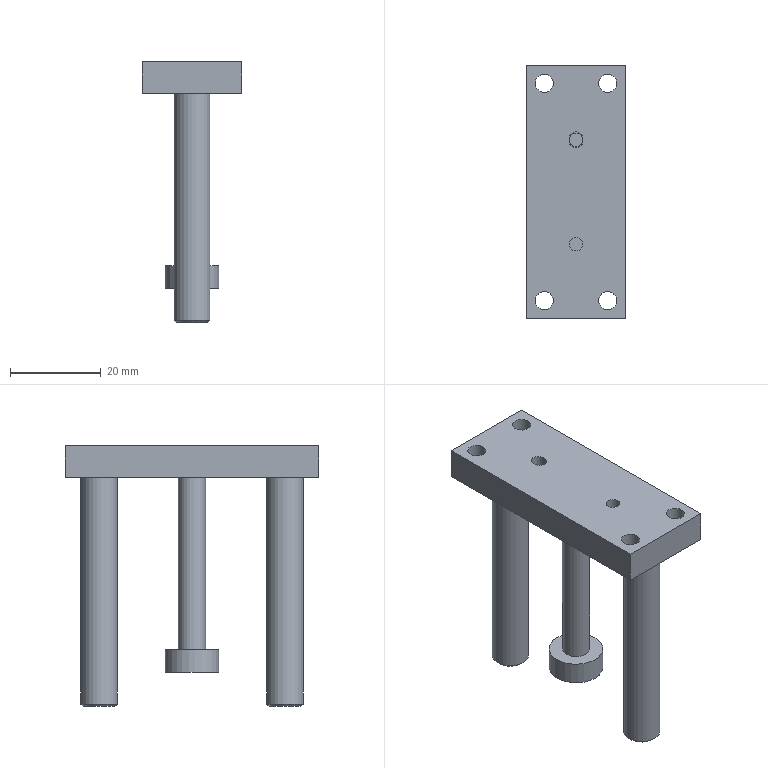Part | STEP file | ROTATION MC_NEW VER-0610_495 | 1 solid | 30 faces | box 22 x 56 x 57.5 mm | volume 14884 mm3 | plane 16 | cylinder 12 | cone 2 | commonest cylinder face diameters 3 x4 4 x4 8 x2 6 x1 11.9 x1
STEP:
#1=CARTESIAN_POINT('',(402.531,450.468,-69.091));
#2=VERTEX_POINT('',#1);
#3=CARTESIAN_POINT('',(380.531,450.468,-69.091));
#4=VERTEX_POINT('',#3);
#5=CARTESIAN_POINT('',(402.531,450.468,-69.091));
#6=DIRECTION('',(-1.,0.,0.));
#7=VECTOR('',#6,22.);
#8=LINE('',#5,#7);
#9=EDGE_CURVE('',#2,#4,#8,.T.);
#10=ORIENTED_EDGE('',*,*,#9,.T.);
#11=CARTESIAN_POINT('',(380.531,450.468,-62.091));
#12=VERTEX_POINT('',#11);
#13=CARTESIAN_POINT('',(380.531,450.468,-62.091));
#14=DIRECTION('',(0.,0.,-1.));
#15=VECTOR('',#14,7.);
#16=LINE('',#13,#15);
#17=EDGE_CURVE('',#12,#4,#16,.T.);
#18=ORIENTED_EDGE('',*,*,#17,.F.);
#19=CARTESIAN_POINT('',(402.531,450.468,-62.091));
#20=VERTEX_POINT('',#19);
#21=CARTESIAN_POINT('',(402.531,450.468,-62.091));
#22=DIRECTION('',(-1.,0.,0.));
#23=VECTOR('',#22,22.);
#24=LINE('',#21,#23);
#25=EDGE_CURVE('',#20,#12,#24,.T.);
#26=ORIENTED_EDGE('',*,*,#25,.F.);
#27=CARTESIAN_POINT('',(402.531,450.468,-62.091));
#28=DIRECTION('',(0.,0.,-1.));
#29=VECTOR('',#28,7.);
#30=LINE('',#27,#29);
#31=EDGE_CURVE('',#20,#2,#30,.T.);
#32=ORIENTED_EDGE('',*,*,#31,.T.);
#33=EDGE_LOOP('',(#10,#18,#26,#32));
#34=FACE_OUTER_BOUND('',#33,.T.);
#35=CARTESIAN_POINT('',(402.531,450.468,-62.091));
#36=DIRECTION('',(0.,-1.,0.));
#37=DIRECTION('',(0.,0.,-1.));
#38=AXIS2_PLACEMENT_3D('',#35,#36,#37);
#39=PLANE('',#38);
#40=ADVANCED_FACE('',(#34),#39,.F.);
#41=CARTESIAN_POINT('',(380.531,394.468,-69.091));
#42=VERTEX_POINT('',#41);
#43=CARTESIAN_POINT('',(380.531,450.468,-69.091));
#44=DIRECTION('',(0.,-1.,0.));
#45=VECTOR('',#44,56.);
#46=LINE('',#43,#45);
#47=EDGE_CURVE('',#4,#42,#46,.T.);
#48=ORIENTED_EDGE('',*,*,#47,.T.);
#49=CARTESIAN_POINT('',(380.531,394.468,-62.091));
#50=VERTEX_POINT('',#49);
#51=CARTESIAN_POINT('',(380.531,394.468,-62.091));
#52=DIRECTION('',(0.,0.,-1.));
#53=VECTOR('',#52,7.);
#54=LINE('',#51,#53);
#55=EDGE_CURVE('',#50,#42,#54,.T.);
#56=ORIENTED_EDGE('',*,*,#55,.F.);
#57=CARTESIAN_POINT('',(380.531,450.468,-62.091));
#58=DIRECTION('',(0.,-1.,0.));
#59=VECTOR('',#58,56.);
#60=LINE('',#57,#59);
#61=EDGE_CURVE('',#12,#50,#60,.T.);
#62=ORIENTED_EDGE('',*,*,#61,.F.);
#63=ORIENTED_EDGE('',*,*,#17,.T.);
#64=EDGE_LOOP('',(#48,#56,#62,#63));
#65=FACE_OUTER_BOUND('',#64,.T.);
#66=CARTESIAN_POINT('',(380.531,450.468,-62.091));
#67=DIRECTION('',(1.,0.,0.));
#68=DIRECTION('',(0.,0.,-1.));
#69=AXIS2_PLACEMENT_3D('',#66,#67,#68);
#70=PLANE('',#69);
#71=ADVANCED_FACE('',(#65),#70,.F.);
#72=CARTESIAN_POINT('',(402.531,394.468,-69.091));
#73=VERTEX_POINT('',#72);
#74=CARTESIAN_POINT('',(380.531,394.468,-69.091));
#75=DIRECTION('',(1.,0.,0.));
#76=VECTOR('',#75,22.);
#77=LINE('',#74,#76);
#78=EDGE_CURVE('',#42,#73,#77,.T.);
#79=ORIENTED_EDGE('',*,*,#78,.T.);
#80=CARTESIAN_POINT('',(402.531,394.468,-62.091));
#81=VERTEX_POINT('',#80);
#82=CARTESIAN_POINT('',(402.531,394.468,-62.091));
#83=DIRECTION('',(0.,0.,-1.));
#84=VECTOR('',#83,7.);
#85=LINE('',#82,#84);
#86=EDGE_CURVE('',#81,#73,#85,.T.);
#87=ORIENTED_EDGE('',*,*,#86,.F.);
#88=CARTESIAN_POINT('',(380.531,394.468,-62.091));
#89=DIRECTION('',(1.,0.,0.));
#90=VECTOR('',#89,22.);
#91=LINE('',#88,#90);
#92=EDGE_CURVE('',#50,#81,#91,.T.);
#93=ORIENTED_EDGE('',*,*,#92,.F.);
#94=ORIENTED_EDGE('',*,*,#55,.T.);
#95=EDGE_LOOP('',(#79,#87,#93,#94));
#96=FACE_OUTER_BOUND('',#95,.T.);
#97=CARTESIAN_POINT('',(402.531,394.468,-62.091));
#98=DIRECTION('',(0.,1.,0.));
#99=DIRECTION('',(0.,0.,1.));
#100=AXIS2_PLACEMENT_3D('',#97,#98,#99);
#101=PLANE('',#100);
#102=ADVANCED_FACE('',(#96),#101,.F.);
#103=CARTESIAN_POINT('',(402.531,394.468,-69.091));
#104=DIRECTION('',(0.,1.,0.));
#105=VECTOR('',#104,56.);
#106=LINE('',#103,#105);
#107=EDGE_CURVE('',#73,#2,#106,.T.);
#108=ORIENTED_EDGE('',*,*,#107,.T.);
#109=ORIENTED_EDGE('',*,*,#31,.F.);
#110=CARTESIAN_POINT('',(402.531,394.468,-62.091));
#111=DIRECTION('',(0.,1.,0.));
#112=VECTOR('',#111,56.);
#113=LINE('',#110,#112);
#114=EDGE_CURVE('',#81,#20,#113,.T.);
#115=ORIENTED_EDGE('',*,*,#114,.F.);
#116=ORIENTED_EDGE('',*,*,#86,.T.);
#117=EDGE_LOOP('',(#108,#109,#115,#116));
#118=FACE_OUTER_BOUND('',#117,.T.);
#119=CARTESIAN_POINT('',(402.531,450.468,-62.091));
#120=DIRECTION('',(-1.,0.,0.));
#121=DIRECTION('',(0.,0.,1.));
#122=AXIS2_PLACEMENT_3D('',#119,#120,#121);
#123=PLANE('',#122);
#124=ADVANCED_FACE('',(#118),#123,.F.);
#125=ORIENTED_EDGE('',*,*,#25,.T.);
#126=ORIENTED_EDGE('',*,*,#61,.T.);
#127=ORIENTED_EDGE('',*,*,#92,.T.);
#128=ORIENTED_EDGE('',*,*,#114,.T.);
#129=EDGE_LOOP('',(#125,#126,#127,#128));
#130=FACE_OUTER_BOUND('',#129,.T.);
#131=CARTESIAN_POINT('',(390.031,433.718,-62.091));
#132=VERTEX_POINT('',#131);
#133=CARTESIAN_POINT('',(393.031,433.718,-62.091));
#134=VERTEX_POINT('',#133);
#135=CARTESIAN_POINT('',(391.531,433.718,-62.091));
#136=DIRECTION('',(0.,0.,1.));
#137=DIRECTION('',(0.,-1.,0.));
#138=AXIS2_PLACEMENT_3D('',#135,#136,#137);
#139=CIRCLE('',#138,1.5);
#140=EDGE_CURVE('',#132,#134,#139,.T.);
#141=ORIENTED_EDGE('',*,*,#140,.F.);
#142=CARTESIAN_POINT('',(390.031,434.218,-62.091));
#143=VERTEX_POINT('',#142);
#144=CARTESIAN_POINT('',(390.031,434.218,-62.091));
#145=DIRECTION('',(0.,-1.,0.));
#146=VECTOR('',#145,0.5);
#147=LINE('',#144,#146);
#148=EDGE_CURVE('',#143,#132,#147,.T.);
#149=ORIENTED_EDGE('',*,*,#148,.F.);
#150=CARTESIAN_POINT('',(393.031,434.218,-62.091));
#151=VERTEX_POINT('',#150);
#152=CARTESIAN_POINT('',(391.531,434.218,-62.091));
#153=DIRECTION('',(0.,0.,1.));
#154=DIRECTION('',(0.,-1.,0.));
#155=AXIS2_PLACEMENT_3D('',#152,#153,#154);
#156=CIRCLE('',#155,1.5);
#157=EDGE_CURVE('',#151,#143,#156,.T.);
#158=ORIENTED_EDGE('',*,*,#157,.F.);
#159=CARTESIAN_POINT('',(393.031,433.718,-62.091));
#160=DIRECTION('',(0.,1.,0.));
#161=VECTOR('',#160,0.5);
#162=LINE('',#159,#161);
#163=EDGE_CURVE('',#134,#151,#162,.T.);
#164=ORIENTED_EDGE('',*,*,#163,.F.);
#165=EDGE_LOOP('',(#141,#149,#158,#164));
#166=FACE_BOUND('',#165,.T.);
#167=CARTESIAN_POINT('',(398.531,448.468,-62.091));
#168=VERTEX_POINT('',#167);
#169=CARTESIAN_POINT('',(398.531,446.468,-62.091));
#170=DIRECTION('',(0.,0.,1.));
#171=DIRECTION('',(0.,1.,0.));
#172=AXIS2_PLACEMENT_3D('',#169,#170,#171);
#173=CIRCLE('',#172,2.);
#174=EDGE_CURVE('',#168,#168,#173,.T.);
#175=ORIENTED_EDGE('',*,*,#174,.F.);
#176=EDGE_LOOP('',(#175));
#177=FACE_BOUND('',#176,.T.);
#178=CARTESIAN_POINT('',(384.531,396.468,-62.091));
#179=VERTEX_POINT('',#178);
#180=CARTESIAN_POINT('',(384.531,400.468,-62.091));
#181=VERTEX_POINT('',#180);
#182=CARTESIAN_POINT('',(384.531,398.468,-62.091));
#183=DIRECTION('',(0.,0.,1.));
#184=DIRECTION('',(0.,-1.,0.));
#185=AXIS2_PLACEMENT_3D('',#182,#183,#184);
#186=CIRCLE('',#185,2.);
#187=EDGE_CURVE('',#179,#181,#186,.T.);
#188=ORIENTED_EDGE('',*,*,#187,.F.);
#189=CARTESIAN_POINT('',(384.531,398.468,-62.091));
#190=DIRECTION('',(0.,0.,1.));
#191=DIRECTION('',(0.,-1.,0.));
#192=AXIS2_PLACEMENT_3D('',#189,#190,#191);
#193=CIRCLE('',#192,2.);
#194=EDGE_CURVE('',#181,#179,#193,.T.);
#195=ORIENTED_EDGE('',*,*,#194,.F.);
#196=EDGE_LOOP('',(#188,#195));
#197=FACE_BOUND('',#196,.T.);
#198=CARTESIAN_POINT('',(384.531,448.468,-62.091));
#199=VERTEX_POINT('',#198);
#200=CARTESIAN_POINT('',(384.531,446.468,-62.091));
#201=DIRECTION('',(0.,0.,1.));
#202=DIRECTION('',(0.,1.,0.));
#203=AXIS2_PLACEMENT_3D('',#200,#201,#202);
#204=CIRCLE('',#203,2.);
#205=EDGE_CURVE('',#199,#199,#204,.T.);
#206=ORIENTED_EDGE('',*,*,#205,.F.);
#207=EDGE_LOOP('',(#206));
#208=FACE_BOUND('',#207,.T.);
#209=CARTESIAN_POINT('',(398.531,396.468,-62.091));
#210=VERTEX_POINT('',#209);
#211=CARTESIAN_POINT('',(398.531,400.468,-62.091));
#212=VERTEX_POINT('',#211);
#213=CARTESIAN_POINT('',(398.531,398.468,-62.091));
#214=DIRECTION('',(0.,0.,1.));
#215=DIRECTION('',(0.,-1.,0.));
#216=AXIS2_PLACEMENT_3D('',#213,#214,#215);
#217=CIRCLE('',#216,2.);
#218=EDGE_CURVE('',#210,#212,#217,.T.);
#219=ORIENTED_EDGE('',*,*,#218,.F.);
#220=CARTESIAN_POINT('',(398.531,398.468,-62.091));
#221=DIRECTION('',(0.,0.,1.));
#222=DIRECTION('',(0.,-1.,0.));
#223=AXIS2_PLACEMENT_3D('',#220,#221,#222);
#224=CIRCLE('',#223,2.);
#225=EDGE_CURVE('',#212,#210,#224,.T.);
#226=ORIENTED_EDGE('',*,*,#225,.F.);
#227=EDGE_LOOP('',(#219,#226));
#228=FACE_BOUND('',#227,.T.);
#229=CARTESIAN_POINT('',(391.531,409.468,-62.091));
#230=VERTEX_POINT('',#229);
#231=CARTESIAN_POINT('',(391.531,412.468,-62.091));
#232=VERTEX_POINT('',#231);
#233=CARTESIAN_POINT('',(391.531,410.968,-62.091));
#234=DIRECTION('',(0.,0.,1.));
#235=DIRECTION('',(0.,-1.,0.));
#236=AXIS2_PLACEMENT_3D('',#233,#234,#235);
#237=CIRCLE('',#236,1.5);
#238=EDGE_CURVE('',#230,#232,#237,.T.);
#239=ORIENTED_EDGE('',*,*,#238,.F.);
#240=CARTESIAN_POINT('',(391.531,410.968,-62.091));
#241=DIRECTION('',(0.,0.,1.));
#242=DIRECTION('',(0.,-1.,0.));
#243=AXIS2_PLACEMENT_3D('',#240,#241,#242);
#244=CIRCLE('',#243,1.5);
#245=EDGE_CURVE('',#232,#230,#244,.T.);
#246=ORIENTED_EDGE('',*,*,#245,.F.);
#247=EDGE_LOOP('',(#239,#246));
#248=FACE_BOUND('',#247,.T.);
#249=CARTESIAN_POINT('',(380.531,450.468,-62.091));
#250=DIRECTION('',(0.,0.,1.));
#251=DIRECTION('',(1.,0.,0.));
#252=AXIS2_PLACEMENT_3D('',#249,#250,#251);
#253=PLANE('',#252);
#254=ADVANCED_FACE('',(#130,#166,#177,#197,#208,#228,#248),#253,.T.);
#255=ORIENTED_EDGE('',*,*,#9,.F.);
#256=ORIENTED_EDGE('',*,*,#107,.F.);
#257=ORIENTED_EDGE('',*,*,#78,.F.);
#258=ORIENTED_EDGE('',*,*,#47,.F.);
#259=EDGE_LOOP('',(#255,#256,#257,#258));
#260=FACE_OUTER_BOUND('',#259,.T.);
#261=CARTESIAN_POINT('',(398.531,444.468,-69.091));
#262=VERTEX_POINT('',#261);
#263=CARTESIAN_POINT('',(398.531,448.468,-69.091));
#264=VERTEX_POINT('',#263);
#265=CARTESIAN_POINT('',(398.531,446.468,-69.091));
#266=DIRECTION('',(0.,0.,1.));
#267=DIRECTION('',(0.,-1.,0.));
#268=AXIS2_PLACEMENT_3D('',#265,#266,#267);
#269=CIRCLE('',#268,2.);
#270=EDGE_CURVE('',#262,#264,#269,.T.);
#271=ORIENTED_EDGE('',*,*,#270,.T.);
#272=CARTESIAN_POINT('',(398.531,446.468,-69.091));
#273=DIRECTION('',(0.,0.,1.));
#274=DIRECTION('',(0.,-1.,0.));
#275=AXIS2_PLACEMENT_3D('',#272,#273,#274);
#276=CIRCLE('',#275,2.);
#277=EDGE_CURVE('',#264,#262,#276,.T.);
#278=ORIENTED_EDGE('',*,*,#277,.T.);
#279=EDGE_LOOP('',(#271,#278));
#280=FACE_BOUND('',#279,.T.);
#281=CARTESIAN_POINT('',(384.531,396.468,-69.091));
#282=VERTEX_POINT('',#281);
#283=CARTESIAN_POINT('',(384.531,400.468,-69.091));
#284=VERTEX_POINT('',#283);
#285=CARTESIAN_POINT('',(384.531,398.468,-69.091));
#286=DIRECTION('',(0.,0.,1.));
#287=DIRECTION('',(0.,-1.,0.));
#288=AXIS2_PLACEMENT_3D('',#285,#286,#287);
#289=CIRCLE('',#288,2.);
#290=EDGE_CURVE('',#282,#284,#289,.T.);
#291=ORIENTED_EDGE('',*,*,#290,.T.);
#292=CARTESIAN_POINT('',(384.531,398.468,-69.091));
#293=DIRECTION('',(0.,0.,1.));
#294=DIRECTION('',(0.,-1.,0.));
#295=AXIS2_PLACEMENT_3D('',#292,#293,#294);
#296=CIRCLE('',#295,2.);
#297=EDGE_CURVE('',#284,#282,#296,.T.);
#298=ORIENTED_EDGE('',*,*,#297,.T.);
#299=EDGE_LOOP('',(#291,#298));
#300=FACE_BOUND('',#299,.T.);
#301=CARTESIAN_POINT('',(384.531,444.468,-69.091));
#302=VERTEX_POINT('',#301);
#303=CARTESIAN_POINT('',(384.531,448.468,-69.091));
#304=VERTEX_POINT('',#303);
#305=CARTESIAN_POINT('',(384.531,446.468,-69.091));
#306=DIRECTION('',(0.,0.,1.));
#307=DIRECTION('',(0.,-1.,0.));
#308=AXIS2_PLACEMENT_3D('',#305,#306,#307);
#309=CIRCLE('',#308,2.);
#310=EDGE_CURVE('',#302,#304,#309,.T.);
#311=ORIENTED_EDGE('',*,*,#310,.T.);
#312=CARTESIAN_POINT('',(384.531,446.468,-69.091));
#313=DIRECTION('',(0.,0.,1.));
#314=DIRECTION('',(0.,-1.,0.));
#315=AXIS2_PLACEMENT_3D('',#312,#313,#314);
#316=CIRCLE('',#315,2.);
#317=EDGE_CURVE('',#304,#302,#316,.T.);
#318=ORIENTED_EDGE('',*,*,#317,.T.);
#319=EDGE_LOOP('',(#311,#318));
#320=FACE_BOUND('',#319,.T.);
#321=CARTESIAN_POINT('',(398.531,396.468,-69.091));
#322=VERTEX_POINT('',#321);
#323=CARTESIAN_POINT('',(398.531,400.468,-69.091));
#324=VERTEX_POINT('',#323);
#325=CARTESIAN_POINT('',(398.531,398.468,-69.091));
#326=DIRECTION('',(0.,0.,1.));
#327=DIRECTION('',(0.,-1.,0.));
#328=AXIS2_PLACEMENT_3D('',#325,#326,#327);
#329=CIRCLE('',#328,2.);
#330=EDGE_CURVE('',#322,#324,#329,.T.);
#331=ORIENTED_EDGE('',*,*,#330,.T.);
#332=CARTESIAN_POINT('',(398.531,398.468,-69.091));
#333=DIRECTION('',(0.,0.,1.));
#334=DIRECTION('',(0.,-1.,0.));
#335=AXIS2_PLACEMENT_3D('',#332,#333,#334);
#336=CIRCLE('',#335,2.);
#337=EDGE_CURVE('',#324,#322,#336,.T.);
#338=ORIENTED_EDGE('',*,*,#337,.T.);
#339=EDGE_LOOP('',(#331,#338));
#340=FACE_BOUND('',#339,.T.);
#341=CARTESIAN_POINT('',(391.531,438.968,-69.091));
#342=VERTEX_POINT('',#341);
#343=CARTESIAN_POINT('',(391.531,446.968,-69.091));
#344=VERTEX_POINT('',#343);
#345=CARTESIAN_POINT('',(391.531,442.968,-69.091));
#346=DIRECTION('',(0.,0.,1.));
#347=DIRECTION('',(0.,-1.,0.));
#348=AXIS2_PLACEMENT_3D('',#345,#346,#347);
#349=CIRCLE('',#348,4.);
#350=EDGE_CURVE('',#342,#344,#349,.F.);
#351=ORIENTED_EDGE('',*,*,#350,.F.);
#352=CARTESIAN_POINT('',(391.531,442.968,-69.091));
#353=DIRECTION('',(0.,0.,1.));
#354=DIRECTION('',(0.,-1.,0.));
#355=AXIS2_PLACEMENT_3D('',#352,#353,#354);
#356=CIRCLE('',#355,4.);
#357=EDGE_CURVE('',#344,#342,#356,.F.);
#358=ORIENTED_EDGE('',*,*,#357,.F.);
#359=EDGE_LOOP('',(#351,#358));
#360=FACE_BOUND('',#359,.T.);
#361=CARTESIAN_POINT('',(391.531,397.968,-69.091));
#362=VERTEX_POINT('',#361);
#363=CARTESIAN_POINT('',(391.531,405.968,-69.091));
#364=VERTEX_POINT('',#363);
#365=CARTESIAN_POINT('',(391.531,401.968,-69.091));
#366=DIRECTION('',(0.,0.,1.));
#367=DIRECTION('',(0.,-1.,0.));
#368=AXIS2_PLACEMENT_3D('',#365,#366,#367);
#369=CIRCLE('',#368,4.);
#370=EDGE_CURVE('',#362,#364,#369,.F.);
#371=ORIENTED_EDGE('',*,*,#370,.F.);
#372=CARTESIAN_POINT('',(391.531,401.968,-69.091));
#373=DIRECTION('',(0.,0.,1.));
#374=DIRECTION('',(0.,-1.,0.));
#375=AXIS2_PLACEMENT_3D('',#372,#373,#374);
#376=CIRCLE('',#375,4.);
#377=EDGE_CURVE('',#364,#362,#376,.F.);
#378=ORIENTED_EDGE('',*,*,#377,.F.);
#379=EDGE_LOOP('',(#371,#378));
#380=FACE_BOUND('',#379,.T.);
#381=CARTESIAN_POINT('',(391.531,419.468,-69.091));
#382=VERTEX_POINT('',#381);
#383=CARTESIAN_POINT('',(391.531,425.468,-69.091));
#384=VERTEX_POINT('',#383);
#385=CARTESIAN_POINT('',(391.531,422.468,-69.091));
#386=DIRECTION('',(0.,0.,1.));
#387=DIRECTION('',(0.,-1.,0.));
#388=AXIS2_PLACEMENT_3D('',#385,#386,#387);
#389=CIRCLE('',#388,3.);
#390=EDGE_CURVE('',#382,#384,#389,.T.);
#391=ORIENTED_EDGE('',*,*,#390,.T.);
#392=CARTESIAN_POINT('',(391.531,422.468,-69.091));
#393=DIRECTION('',(0.,0.,1.));
#394=DIRECTION('',(0.,-1.,0.));
#395=AXIS2_PLACEMENT_3D('',#392,#393,#394);
#396=CIRCLE('',#395,3.);
#397=EDGE_CURVE('',#384,#382,#396,.T.);
#398=ORIENTED_EDGE('',*,*,#397,.T.);
#399=EDGE_LOOP('',(#391,#398));
#400=FACE_BOUND('',#399,.T.);
#401=CARTESIAN_POINT('',(380.531,450.468,-69.091));
#402=DIRECTION('',(0.,0.,1.));
#403=DIRECTION('',(1.,0.,0.));
#404=AXIS2_PLACEMENT_3D('',#401,#402,#403);
#405=PLANE('',#404);
#406=ADVANCED_FACE('',(#260,#280,#300,#320,#340,#360,#380,#400),#405,.F.);
#407=ORIENTED_EDGE('',*,*,#390,.F.);
#408=ORIENTED_EDGE('',*,*,#397,.F.);
#409=CARTESIAN_POINT('',(391.531,425.468,-107.091));
#410=VERTEX_POINT('',#409);
#411=CARTESIAN_POINT('',(391.531,425.468,-120.577));
#412=DIRECTION('',(0.,0.,-1.));
#413=VECTOR('',#412,3.);
#414=LINE('',#411,#413);
#415=EDGE_CURVE('',#384,#410,#414,.T.);
#416=ORIENTED_EDGE('',*,*,#415,.T.);
#417=CARTESIAN_POINT('',(391.531,419.468,-107.091));
#418=VERTEX_POINT('',#417);
#419=CARTESIAN_POINT('',(391.531,422.468,-107.091));
#420=DIRECTION('',(0.,0.,1.));
#421=DIRECTION('',(0.,-1.,0.));
#422=AXIS2_PLACEMENT_3D('',#419,#420,#421);
#423=CIRCLE('',#422,3.);
#424=EDGE_CURVE('',#418,#410,#423,.F.);
#425=ORIENTED_EDGE('',*,*,#424,.F.);
#426=CARTESIAN_POINT('',(391.531,422.468,-107.091));
#427=DIRECTION('',(0.,0.,1.));
#428=DIRECTION('',(0.,-1.,0.));
#429=AXIS2_PLACEMENT_3D('',#426,#427,#428);
#430=CIRCLE('',#429,3.);
#431=EDGE_CURVE('',#410,#418,#430,.F.);
#432=ORIENTED_EDGE('',*,*,#431,.F.);
#433=ORIENTED_EDGE('',*,*,#415,.F.);
#434=EDGE_LOOP('',(#407,#408,#416,#425,#432,#433));
#435=FACE_OUTER_BOUND('',#434,.T.);
#436=CARTESIAN_POINT('',(391.531,422.468,-120.577));
#437=DIRECTION('',(0.,0.,1.));
#438=DIRECTION('',(0.,-1.,0.));
#439=AXIS2_PLACEMENT_3D('',#436,#437,#438);
#440=CYLINDRICAL_SURFACE('',#439,3.);
#441=ADVANCED_FACE('',(#435),#440,.T.);
#442=CARTESIAN_POINT('',(391.531,416.518,-112.091));
#443=VERTEX_POINT('',#442);
#444=CARTESIAN_POINT('',(391.531,422.468,-112.091));
#445=DIRECTION('',(0.,0.,1.));
#446=DIRECTION('',(0.,-1.,0.));
#447=AXIS2_PLACEMENT_3D('',#444,#445,#446);
#448=CIRCLE('',#447,5.95);
#449=EDGE_CURVE('',#443,#443,#448,.T.);
#450=ORIENTED_EDGE('',*,*,#449,.T.);
#451=CARTESIAN_POINT('',(391.531,416.518,-107.091));
#452=VERTEX_POINT('',#451);
#453=CARTESIAN_POINT('',(391.531,416.518,-107.091));
#454=DIRECTION('',(0.,0.,1.));
#455=VECTOR('',#454,5.95);
#456=LINE('',#453,#455);
#457=EDGE_CURVE('',#443,#452,#456,.T.);
#458=ORIENTED_EDGE('',*,*,#457,.T.);
#459=CARTESIAN_POINT('',(391.531,422.468,-107.091));
#460=DIRECTION('',(0.,0.,1.));
#461=DIRECTION('',(0.,-1.,0.));
#462=AXIS2_PLACEMENT_3D('',#459,#460,#461);
#463=CIRCLE('',#462,5.95);
#464=EDGE_CURVE('',#452,#452,#463,.T.);
#465=ORIENTED_EDGE('',*,*,#464,.F.);
#466=ORIENTED_EDGE('',*,*,#457,.F.);
#467=EDGE_LOOP('',(#450,#458,#465,#466));
#468=FACE_OUTER_BOUND('',#467,.T.);
#469=CARTESIAN_POINT('',(391.531,422.468,-107.091));
#470=DIRECTION('',(0.,0.,-1.));
#471=DIRECTION('',(0.,1.,0.));
#472=AXIS2_PLACEMENT_3D('',#469,#470,#471);
#473=CYLINDRICAL_SURFACE('',#472,5.95);
#474=ADVANCED_FACE('',(#468),#473,.T.);
#475=ORIENTED_EDGE('',*,*,#464,.T.);
#476=EDGE_LOOP('',(#475));
#477=FACE_OUTER_BOUND('',#476,.T.);
#478=ORIENTED_EDGE('',*,*,#424,.T.);
#479=ORIENTED_EDGE('',*,*,#431,.T.);
#480=EDGE_LOOP('',(#478,#479));
#481=FACE_BOUND('',#480,.T.);
#482=CARTESIAN_POINT('',(391.531,422.468,-107.091));
#483=DIRECTION('',(0.,0.,1.));
#484=DIRECTION('',(1.,0.,0.));
#485=AXIS2_PLACEMENT_3D('',#482,#483,#484);
#486=PLANE('',#485);
#487=ADVANCED_FACE('',(#477,#481),#486,.T.);
#488=ORIENTED_EDGE('',*,*,#449,.F.);
#489=EDGE_LOOP('',(#488));
#490=FACE_OUTER_BOUND('',#489,.T.);
#491=CARTESIAN_POINT('',(391.531,422.468,-112.091));
#492=DIRECTION('',(0.,0.,1.));
#493=DIRECTION('',(1.,0.,0.));
#494=AXIS2_PLACEMENT_3D('',#491,#492,#493);
#495=PLANE('',#494);
#496=ADVANCED_FACE('',(#490),#495,.F.);
#497=ORIENTED_EDGE('',*,*,#370,.T.);
#498=CARTESIAN_POINT('',(391.531,405.968,-119.091));
#499=VERTEX_POINT('',#498);
#500=CARTESIAN_POINT('',(391.531,405.968,-130.905));
#501=DIRECTION('',(0.,0.,-1.));
#502=VECTOR('',#501,4.);
#503=LINE('',#500,#502);
#504=EDGE_CURVE('',#364,#499,#503,.T.);
#505=ORIENTED_EDGE('',*,*,#504,.T.);
#506=CARTESIAN_POINT('',(391.531,397.968,-119.091));
#507=VERTEX_POINT('',#506);
#508=CARTESIAN_POINT('',(391.531,401.968,-119.091));
#509=DIRECTION('',(0.,0.,1.));
#510=DIRECTION('',(0.,-1.,0.));
#511=AXIS2_PLACEMENT_3D('',#508,#509,#510);
#512=CIRCLE('',#511,4.);
#513=EDGE_CURVE('',#499,#507,#512,.T.);
#514=ORIENTED_EDGE('',*,*,#513,.T.);
#515=CARTESIAN_POINT('',(391.531,401.968,-119.091));
#516=DIRECTION('',(0.,0.,1.));
#517=DIRECTION('',(0.,-1.,0.));
#518=AXIS2_PLACEMENT_3D('',#515,#516,#517);
#519=CIRCLE('',#518,4.);
#520=EDGE_CURVE('',#507,#499,#519,.T.);
#521=ORIENTED_EDGE('',*,*,#520,.T.);
#522=ORIENTED_EDGE('',*,*,#504,.F.);
#523=ORIENTED_EDGE('',*,*,#377,.T.);
#524=EDGE_LOOP('',(#497,#505,#514,#521,#522,#523));
#525=FACE_OUTER_BOUND('',#524,.T.);
#526=CARTESIAN_POINT('',(391.531,401.968,-130.905));
#527=DIRECTION('',(0.,0.,1.));
#528=DIRECTION('',(0.,-1.,0.));
#529=AXIS2_PLACEMENT_3D('',#526,#527,#528);
#530=CYLINDRICAL_SURFACE('',#529,4.);
#531=ADVANCED_FACE('',(#525),#530,.T.);
#532=CARTESIAN_POINT('',(391.531,398.468,-119.591));
#533=VERTEX_POINT('',#532);
#534=CARTESIAN_POINT('',(391.531,405.468,-119.591));
#535=VERTEX_POINT('',#534);
#536=CARTESIAN_POINT('',(391.531,401.968,-119.591));
#537=DIRECTION('',(0.,0.,1.));
#538=DIRECTION('',(0.,-1.,0.));
#539=AXIS2_PLACEMENT_3D('',#536,#537,#538);
#540=CIRCLE('',#539,3.5);
#541=EDGE_CURVE('',#533,#535,#540,.F.);
#542=ORIENTED_EDGE('',*,*,#541,.T.);
#543=CARTESIAN_POINT('',(391.531,401.968,-119.591));
#544=DIRECTION('',(0.,0.,1.));
#545=DIRECTION('',(0.,-1.,0.));
#546=AXIS2_PLACEMENT_3D('',#543,#544,#545);
#547=CIRCLE('',#546,3.5);
#548=EDGE_CURVE('',#535,#533,#547,.F.);
#549=ORIENTED_EDGE('',*,*,#548,.T.);
#550=EDGE_LOOP('',(#542,#549));
#551=FACE_OUTER_BOUND('',#550,.T.);
#552=CARTESIAN_POINT('',(391.531,422.468,-119.591));
#553=DIRECTION('',(0.,0.,1.));
#554=DIRECTION('',(1.,0.,0.));
#555=AXIS2_PLACEMENT_3D('',#552,#553,#554);
#556=PLANE('',#555);
#557=ADVANCED_FACE('',(#551),#556,.F.);
#558=ORIENTED_EDGE('',*,*,#350,.T.);
#559=CARTESIAN_POINT('',(391.531,446.968,-119.091));
#560=VERTEX_POINT('',#559);
#561=CARTESIAN_POINT('',(391.531,446.968,-130.905));
#562=DIRECTION('',(0.,0.,-1.));
#563=VECTOR('',#562,4.);
#564=LINE('',#561,#563);
#565=EDGE_CURVE('',#344,#560,#564,.T.);
#566=ORIENTED_EDGE('',*,*,#565,.T.);
#567=CARTESIAN_POINT('',(391.531,438.968,-119.091));
#568=VERTEX_POINT('',#567);
#569=CARTESIAN_POINT('',(391.531,442.968,-119.091));
#570=DIRECTION('',(0.,0.,1.));
#571=DIRECTION('',(0.,-1.,0.));
#572=AXIS2_PLACEMENT_3D('',#569,#570,#571);
#573=CIRCLE('',#572,4.);
#574=EDGE_CURVE('',#560,#568,#573,.T.);
#575=ORIENTED_EDGE('',*,*,#574,.T.);
#576=CARTESIAN_POINT('',(391.531,442.968,-119.091));
#577=DIRECTION('',(0.,0.,1.));
#578=DIRECTION('',(0.,-1.,0.));
#579=AXIS2_PLACEMENT_3D('',#576,#577,#578);
#580=CIRCLE('',#579,4.);
#581=EDGE_CURVE('',#568,#560,#580,.T.);
#582=ORIENTED_EDGE('',*,*,#581,.T.);
#583=ORIENTED_EDGE('',*,*,#565,.F.);
#584=ORIENTED_EDGE('',*,*,#357,.T.);
#585=EDGE_LOOP('',(#558,#566,#575,#582,#583,#584));
#586=FACE_OUTER_BOUND('',#585,.T.);
#587=CARTESIAN_POINT('',(391.531,442.968,-130.905));
#588=DIRECTION('',(0.,0.,1.));
#589=DIRECTION('',(0.,-1.,0.));
#590=AXIS2_PLACEMENT_3D('',#587,#588,#589);
#591=CYLINDRICAL_SURFACE('',#590,4.);
#592=ADVANCED_FACE('',(#586),#591,.T.);
#593=CARTESIAN_POINT('',(391.531,439.468,-119.591));
#594=VERTEX_POINT('',#593);
#595=CARTESIAN_POINT('',(391.531,446.468,-119.591));
#596=VERTEX_POINT('',#595);
#597=CARTESIAN_POINT('',(391.531,442.968,-119.591));
#598=DIRECTION('',(0.,0.,1.));
#599=DIRECTION('',(0.,-1.,0.));
#600=AXIS2_PLACEMENT_3D('',#597,#598,#599);
#601=CIRCLE('',#600,3.5);
#602=EDGE_CURVE('',#594,#596,#601,.F.);
#603=ORIENTED_EDGE('',*,*,#602,.T.);
#604=CARTESIAN_POINT('',(391.531,442.968,-119.591));
#605=DIRECTION('',(0.,0.,1.));
#606=DIRECTION('',(0.,-1.,0.));
#607=AXIS2_PLACEMENT_3D('',#604,#605,#606);
#608=CIRCLE('',#607,3.5);
#609=EDGE_CURVE('',#596,#594,#608,.F.);
#610=ORIENTED_EDGE('',*,*,#609,.T.);
#611=EDGE_LOOP('',(#603,#610));
#612=FACE_OUTER_BOUND('',#611,.T.);
#613=CARTESIAN_POINT('',(391.531,422.468,-119.591));
#614=DIRECTION('',(0.,0.,1.));
#615=DIRECTION('',(1.,0.,0.));
#616=AXIS2_PLACEMENT_3D('',#613,#614,#615);
#617=PLANE('',#616);
#618=ADVANCED_FACE('',(#612),#617,.F.);
#619=CARTESIAN_POINT('',(391.531,409.468,-68.091));
#620=VERTEX_POINT('',#619);
#621=CARTESIAN_POINT('',(391.531,412.468,-68.091));
#622=VERTEX_POINT('',#621);
#623=CARTESIAN_POINT('',(391.531,410.968,-68.091));
#624=DIRECTION('',(0.,0.,1.));
#625=DIRECTION('',(0.,-1.,0.));
#626=AXIS2_PLACEMENT_3D('',#623,#624,#625);
#627=CIRCLE('',#626,1.5);
#628=EDGE_CURVE('',#620,#622,#627,.T.);
#629=ORIENTED_EDGE('',*,*,#628,.F.);
#630=CARTESIAN_POINT('',(391.531,410.968,-68.091));
#631=DIRECTION('',(0.,0.,1.));
#632=DIRECTION('',(0.,-1.,0.));
#633=AXIS2_PLACEMENT_3D('',#630,#631,#632);
#634=CIRCLE('',#633,1.5);
#635=EDGE_CURVE('',#622,#620,#634,.T.);
#636=ORIENTED_EDGE('',*,*,#635,.F.);
#637=CARTESIAN_POINT('',(391.531,412.468,-68.091));
#638=DIRECTION('',(0.,0.,1.));
#639=VECTOR('',#638,1.5);
#640=LINE('',#637,#639);
#641=EDGE_CURVE('',#622,#232,#640,.T.);
#642=ORIENTED_EDGE('',*,*,#641,.T.);
#643=ORIENTED_EDGE('',*,*,#245,.T.);
#644=ORIENTED_EDGE('',*,*,#238,.T.);
#645=ORIENTED_EDGE('',*,*,#641,.F.);
#646=EDGE_LOOP('',(#629,#636,#642,#643,#644,#645));
#647=FACE_OUTER_BOUND('',#646,.T.);
#648=CARTESIAN_POINT('',(391.531,410.968,-68.091));
#649=DIRECTION('',(0.,0.,1.));
#650=DIRECTION('',(0.,-1.,0.));
#651=AXIS2_PLACEMENT_3D('',#648,#649,#650);
#652=CYLINDRICAL_SURFACE('',#651,1.5);
#653=ADVANCED_FACE('',(#647),#652,.F.);
#654=ORIENTED_EDGE('',*,*,#628,.T.);
#655=ORIENTED_EDGE('',*,*,#635,.T.);
#656=EDGE_LOOP('',(#654,#655));
#657=FACE_OUTER_BOUND('',#656,.T.);
#658=CARTESIAN_POINT('',(391.531,410.968,-68.091));
#659=DIRECTION('',(0.,0.,1.));
#660=DIRECTION('',(1.,0.,0.));
#661=AXIS2_PLACEMENT_3D('',#658,#659,#660);
#662=PLANE('',#661);
#663=ADVANCED_FACE('',(#657),#662,.T.);
#664=ORIENTED_EDGE('',*,*,#520,.F.);
#665=ORIENTED_EDGE('',*,*,#513,.F.);
#666=CARTESIAN_POINT('',(391.531,405.968,-119.091));
#667=DIRECTION('',(0.,-0.7071,-0.7071));
#668=VECTOR('',#667,4.);
#669=LINE('',#666,#668);
#670=EDGE_CURVE('',#499,#535,#669,.T.);
#671=ORIENTED_EDGE('',*,*,#670,.T.);
#672=ORIENTED_EDGE('',*,*,#541,.F.);
#673=ORIENTED_EDGE('',*,*,#548,.F.);
#674=ORIENTED_EDGE('',*,*,#670,.F.);
#675=EDGE_LOOP('',(#664,#665,#671,#672,#673,#674));
#676=FACE_OUTER_BOUND('',#675,.T.);
#677=CARTESIAN_POINT('',(391.531,401.968,-119.091));
#678=DIRECTION('',(0.,0.,1.));
#679=DIRECTION('',(0.,-1.,0.));
#680=AXIS2_PLACEMENT_3D('',#677,#678,#679);
#681=CONICAL_SURFACE('',#680,4.,0.7854);
#682=ADVANCED_FACE('',(#676),#681,.T.);
#683=ORIENTED_EDGE('',*,*,#581,.F.);
#684=ORIENTED_EDGE('',*,*,#574,.F.);
#685=CARTESIAN_POINT('',(391.531,446.968,-119.091));
#686=DIRECTION('',(0.,-0.7071,-0.7071));
#687=VECTOR('',#686,4.);
#688=LINE('',#685,#687);
#689=EDGE_CURVE('',#560,#596,#688,.T.);
#690=ORIENTED_EDGE('',*,*,#689,.T.);
#691=ORIENTED_EDGE('',*,*,#602,.F.);
#692=ORIENTED_EDGE('',*,*,#609,.F.);
#693=ORIENTED_EDGE('',*,*,#689,.F.);
#694=EDGE_LOOP('',(#683,#684,#690,#691,#692,#693));
#695=FACE_OUTER_BOUND('',#694,.T.);
#696=CARTESIAN_POINT('',(391.531,442.968,-119.091));
#697=DIRECTION('',(0.,0.,1.));
#698=DIRECTION('',(0.,-1.,0.));
#699=AXIS2_PLACEMENT_3D('',#696,#697,#698);
#700=CONICAL_SURFACE('',#699,4.,0.7854);
#701=ADVANCED_FACE('',(#695),#700,.T.);
#702=ORIENTED_EDGE('',*,*,#330,.F.);
#703=ORIENTED_EDGE('',*,*,#337,.F.);
#704=CARTESIAN_POINT('',(398.531,400.468,-119.591));
#705=DIRECTION('',(0.,0.,1.));
#706=VECTOR('',#705,2.);
#707=LINE('',#704,#706);
#708=EDGE_CURVE('',#324,#212,#707,.T.);
#709=ORIENTED_EDGE('',*,*,#708,.T.);
#710=ORIENTED_EDGE('',*,*,#225,.T.);
#711=ORIENTED_EDGE('',*,*,#218,.T.);
#712=ORIENTED_EDGE('',*,*,#708,.F.);
#713=EDGE_LOOP('',(#702,#703,#709,#710,#711,#712));
#714=FACE_OUTER_BOUND('',#713,.T.);
#715=CARTESIAN_POINT('',(398.531,398.468,-119.591));
#716=DIRECTION('',(0.,0.,1.));
#717=DIRECTION('',(0.,-1.,0.));
#718=AXIS2_PLACEMENT_3D('',#715,#716,#717);
#719=CYLINDRICAL_SURFACE('',#718,2.);
#720=ADVANCED_FACE('',(#714),#719,.F.);
#721=ORIENTED_EDGE('',*,*,#310,.F.);
#722=ORIENTED_EDGE('',*,*,#317,.F.);
#723=CARTESIAN_POINT('',(384.531,448.468,-119.591));
#724=DIRECTION('',(0.,0.,1.));
#725=VECTOR('',#724,2.);
#726=LINE('',#723,#725);
#727=EDGE_CURVE('',#304,#199,#726,.T.);
#728=ORIENTED_EDGE('',*,*,#727,.T.);
#729=ORIENTED_EDGE('',*,*,#205,.T.);
#730=ORIENTED_EDGE('',*,*,#727,.F.);
#731=EDGE_LOOP('',(#721,#722,#728,#729,#730));
#732=FACE_OUTER_BOUND('',#731,.T.);
#733=CARTESIAN_POINT('',(384.531,446.468,-119.591));
#734=DIRECTION('',(0.,0.,1.));
#735=DIRECTION('',(0.,-1.,0.));
#736=AXIS2_PLACEMENT_3D('',#733,#734,#735);
#737=CYLINDRICAL_SURFACE('',#736,2.);
#738=ADVANCED_FACE('',(#732),#737,.F.);
#739=ORIENTED_EDGE('',*,*,#290,.F.);
#740=ORIENTED_EDGE('',*,*,#297,.F.);
#741=CARTESIAN_POINT('',(384.531,400.468,-119.591));
#742=DIRECTION('',(0.,0.,1.));
#743=VECTOR('',#742,2.);
#744=LINE('',#741,#743);
#745=EDGE_CURVE('',#284,#181,#744,.T.);
#746=ORIENTED_EDGE('',*,*,#745,.T.);
#747=ORIENTED_EDGE('',*,*,#194,.T.);
#748=ORIENTED_EDGE('',*,*,#187,.T.);
#749=ORIENTED_EDGE('',*,*,#745,.F.);
#750=EDGE_LOOP('',(#739,#740,#746,#747,#748,#749));
#751=FACE_OUTER_BOUND('',#750,.T.);
#752=CARTESIAN_POINT('',(384.531,398.468,-119.591));
#753=DIRECTION('',(0.,0.,1.));
#754=DIRECTION('',(0.,-1.,0.));
#755=AXIS2_PLACEMENT_3D('',#752,#753,#754);
#756=CYLINDRICAL_SURFACE('',#755,2.);
#757=ADVANCED_FACE('',(#751),#756,.F.);
#758=ORIENTED_EDGE('',*,*,#270,.F.);
#759=ORIENTED_EDGE('',*,*,#277,.F.);
#760=CARTESIAN_POINT('',(398.531,448.468,-119.591));
#761=DIRECTION('',(0.,0.,1.));
#762=VECTOR('',#761,2.);
#763=LINE('',#760,#762);
#764=EDGE_CURVE('',#264,#168,#763,.T.);
#765=ORIENTED_EDGE('',*,*,#764,.T.);
#766=ORIENTED_EDGE('',*,*,#174,.T.);
#767=ORIENTED_EDGE('',*,*,#764,.F.);
#768=EDGE_LOOP('',(#758,#759,#765,#766,#767));
#769=FACE_OUTER_BOUND('',#768,.T.);
#770=CARTESIAN_POINT('',(398.531,446.468,-119.591));
#771=DIRECTION('',(0.,0.,1.));
#772=DIRECTION('',(0.,-1.,0.));
#773=AXIS2_PLACEMENT_3D('',#770,#771,#772);
#774=CYLINDRICAL_SURFACE('',#773,2.);
#775=ADVANCED_FACE('',(#769),#774,.F.);
#776=ORIENTED_EDGE('',*,*,#148,.T.);
#777=CARTESIAN_POINT('',(390.031,433.718,-65.091));
#778=VERTEX_POINT('',#777);
#779=CARTESIAN_POINT('',(390.031,433.718,-65.091));
#780=DIRECTION('',(0.,0.,1.));
#781=VECTOR('',#780,3.);
#782=LINE('',#779,#781);
#783=EDGE_CURVE('',#778,#132,#782,.T.);
#784=ORIENTED_EDGE('',*,*,#783,.F.);
#785=CARTESIAN_POINT('',(390.031,433.968,-65.091));
#786=VERTEX_POINT('',#785);
#787=CARTESIAN_POINT('',(390.031,433.968,-65.091));
#788=DIRECTION('',(0.,-1.,0.));
#789=VECTOR('',#788,0.25);
#790=LINE('',#787,#789);
#791=EDGE_CURVE('',#786,#778,#790,.T.);
#792=ORIENTED_EDGE('',*,*,#791,.F.);
#793=CARTESIAN_POINT('',(390.031,434.218,-65.091));
#794=VERTEX_POINT('',#793);
#795=CARTESIAN_POINT('',(390.031,434.218,-65.091));
#796=DIRECTION('',(0.,-1.,0.));
#797=VECTOR('',#796,0.25);
#798=LINE('',#795,#797);
#799=EDGE_CURVE('',#794,#786,#798,.T.);
#800=ORIENTED_EDGE('',*,*,#799,.F.);
#801=CARTESIAN_POINT('',(390.031,434.218,-65.091));
#802=DIRECTION('',(0.,0.,1.));
#803=VECTOR('',#802,3.);
#804=LINE('',#801,#803);
#805=EDGE_CURVE('',#794,#143,#804,.T.);
#806=ORIENTED_EDGE('',*,*,#805,.T.);
#807=EDGE_LOOP('',(#776,#784,#792,#800,#806));
#808=FACE_OUTER_BOUND('',#807,.T.);
#809=CARTESIAN_POINT('',(390.031,434.218,-65.091));
#810=DIRECTION('',(-1.,0.,0.));
#811=DIRECTION('',(0.,0.,1.));
#812=AXIS2_PLACEMENT_3D('',#809,#810,#811);
#813=PLANE('',#812);
#814=ADVANCED_FACE('',(#808),#813,.F.);
#815=ORIENTED_EDGE('',*,*,#163,.T.);
#816=CARTESIAN_POINT('',(393.031,434.218,-65.091));
#817=VERTEX_POINT('',#816);
#818=CARTESIAN_POINT('',(393.031,434.218,-65.091));
#819=DIRECTION('',(0.,0.,1.));
#820=VECTOR('',#819,3.);
#821=LINE('',#818,#820);
#822=EDGE_CURVE('',#817,#151,#821,.T.);
#823=ORIENTED_EDGE('',*,*,#822,.F.);
#824=CARTESIAN_POINT('',(393.031,433.968,-65.091));
#825=VERTEX_POINT('',#824);
#826=CARTESIAN_POINT('',(393.031,433.968,-65.091));
#827=DIRECTION('',(0.,1.,0.));
#828=VECTOR('',#827,0.25);
#829=LINE('',#826,#828);
#830=EDGE_CURVE('',#825,#817,#829,.T.);
#831=ORIENTED_EDGE('',*,*,#830,.F.);
#832=CARTESIAN_POINT('',(393.031,433.718,-65.091));
#833=VERTEX_POINT('',#832);
#834=CARTESIAN_POINT('',(393.031,433.718,-65.091));
#835=DIRECTION('',(0.,1.,0.));
#836=VECTOR('',#835,0.25);
#837=LINE('',#834,#836);
#838=EDGE_CURVE('',#833,#825,#837,.T.);
#839=ORIENTED_EDGE('',*,*,#838,.F.);
#840=CARTESIAN_POINT('',(393.031,433.718,-65.091));
#841=DIRECTION('',(0.,0.,1.));
#842=VECTOR('',#841,3.);
#843=LINE('',#840,#842);
#844=EDGE_CURVE('',#833,#134,#843,.T.);
#845=ORIENTED_EDGE('',*,*,#844,.T.);
#846=EDGE_LOOP('',(#815,#823,#831,#839,#845));
#847=FACE_OUTER_BOUND('',#846,.T.);
#848=CARTESIAN_POINT('',(393.031,434.218,-65.091));
#849=DIRECTION('',(1.,0.,0.));
#850=DIRECTION('',(0.,0.,-1.));
#851=AXIS2_PLACEMENT_3D('',#848,#849,#850);
#852=PLANE('',#851);
#853=ADVANCED_FACE('',(#847),#852,.F.);
#854=CARTESIAN_POINT('',(391.531,435.468,-65.091));
#855=VERTEX_POINT('',#854);
#856=CARTESIAN_POINT('',(391.531,433.968,-65.091));
#857=DIRECTION('',(0.,0.,1.));
#858=DIRECTION('',(0.,-1.,0.));
#859=AXIS2_PLACEMENT_3D('',#856,#857,#858);
#860=CIRCLE('',#859,1.5);
#861=EDGE_CURVE('',#786,#855,#860,.F.);
#862=ORIENTED_EDGE('',*,*,#861,.T.);
#863=CARTESIAN_POINT('',(391.531,433.968,-65.091));
#864=DIRECTION('',(0.,0.,1.));
#865=DIRECTION('',(0.,-1.,0.));
#866=AXIS2_PLACEMENT_3D('',#863,#864,#865);
#867=CIRCLE('',#866,1.5);
#868=EDGE_CURVE('',#855,#825,#867,.F.);
#869=ORIENTED_EDGE('',*,*,#868,.T.);
#870=ORIENTED_EDGE('',*,*,#830,.T.);
#871=CARTESIAN_POINT('',(391.531,434.218,-65.091));
#872=DIRECTION('',(0.,0.,1.));
#873=DIRECTION('',(0.,-1.,0.));
#874=AXIS2_PLACEMENT_3D('',#871,#872,#873);
#875=CIRCLE('',#874,1.5);
#876=EDGE_CURVE('',#817,#794,#875,.T.);
#877=ORIENTED_EDGE('',*,*,#876,.T.);
#878=ORIENTED_EDGE('',*,*,#799,.T.);
#879=EDGE_LOOP('',(#862,#869,#870,#877,#878));
#880=FACE_OUTER_BOUND('',#879,.T.);
#881=CARTESIAN_POINT('',(391.531,433.718,-65.091));
#882=DIRECTION('',(0.,0.,1.));
#883=DIRECTION('',(1.,0.,0.));
#884=AXIS2_PLACEMENT_3D('',#881,#882,#883);
#885=PLANE('',#884);
#886=ADVANCED_FACE('',(#880),#885,.T.);
#887=CARTESIAN_POINT('',(391.531,433.968,-65.091));
#888=DIRECTION('',(0.,0.,1.));
#889=DIRECTION('',(0.,-1.,0.));
#890=AXIS2_PLACEMENT_3D('',#887,#888,#889);
#891=CIRCLE('',#890,1.5);
#892=EDGE_CURVE('',#825,#786,#891,.F.);
#893=ORIENTED_EDGE('',*,*,#892,.T.);
#894=ORIENTED_EDGE('',*,*,#791,.T.);
#895=CARTESIAN_POINT('',(391.531,433.718,-65.091));
#896=DIRECTION('',(0.,0.,1.));
#897=DIRECTION('',(0.,-1.,0.));
#898=AXIS2_PLACEMENT_3D('',#895,#896,#897);
#899=CIRCLE('',#898,1.5);
#900=EDGE_CURVE('',#778,#833,#899,.T.);
#901=ORIENTED_EDGE('',*,*,#900,.T.);
#902=ORIENTED_EDGE('',*,*,#838,.T.);
#903=EDGE_LOOP('',(#893,#894,#901,#902));
#904=FACE_OUTER_BOUND('',#903,.T.);
#905=CARTESIAN_POINT('',(391.531,433.718,-65.091));
#906=DIRECTION('',(0.,0.,1.));
#907=DIRECTION('',(1.,0.,0.));
#908=AXIS2_PLACEMENT_3D('',#905,#906,#907);
#909=PLANE('',#908);
#910=ADVANCED_FACE('',(#904),#909,.T.);
#911=ORIENTED_EDGE('',*,*,#140,.T.);
#912=ORIENTED_EDGE('',*,*,#844,.F.);
#913=ORIENTED_EDGE('',*,*,#900,.F.);
#914=ORIENTED_EDGE('',*,*,#783,.T.);
#915=EDGE_LOOP('',(#911,#912,#913,#914));
#916=FACE_OUTER_BOUND('',#915,.T.);
#917=CARTESIAN_POINT('',(391.531,433.718,-65.091));
#918=DIRECTION('',(0.,0.,1.));
#919=DIRECTION('',(0.,-1.,0.));
#920=AXIS2_PLACEMENT_3D('',#917,#918,#919);
#921=CYLINDRICAL_SURFACE('',#920,1.5);
#922=ADVANCED_FACE('',(#916),#921,.F.);
#923=ORIENTED_EDGE('',*,*,#157,.T.);
#924=ORIENTED_EDGE('',*,*,#805,.F.);
#925=ORIENTED_EDGE('',*,*,#876,.F.);
#926=ORIENTED_EDGE('',*,*,#822,.T.);
#927=EDGE_LOOP('',(#923,#924,#925,#926));
#928=FACE_OUTER_BOUND('',#927,.T.);
#929=CARTESIAN_POINT('',(391.531,434.218,-65.091));
#930=DIRECTION('',(0.,0.,1.));
#931=DIRECTION('',(0.,1.,0.));
#932=AXIS2_PLACEMENT_3D('',#929,#930,#931);
#933=CYLINDRICAL_SURFACE('',#932,1.5);
#934=ADVANCED_FACE('',(#928),#933,.F.);
#935=CARTESIAN_POINT('',(391.531,435.468,-68.091));
#936=VERTEX_POINT('',#935);
#937=CARTESIAN_POINT('',(391.531,433.968,-68.091));
#938=DIRECTION('',(0.,0.,1.));
#939=DIRECTION('',(0.,1.,0.));
#940=AXIS2_PLACEMENT_3D('',#937,#938,#939);
#941=CIRCLE('',#940,1.5);
#942=EDGE_CURVE('',#936,#936,#941,.T.);
#943=ORIENTED_EDGE('',*,*,#942,.T.);
#944=EDGE_LOOP('',(#943));
#945=FACE_OUTER_BOUND('',#944,.T.);
#946=CARTESIAN_POINT('',(391.531,433.968,-68.091));
#947=DIRECTION('',(0.,0.,-1.));
#948=DIRECTION('',(-1.,0.,0.));
#949=AXIS2_PLACEMENT_3D('',#946,#947,#948);
#950=PLANE('',#949);
#951=ADVANCED_FACE('',(#945),#950,.F.);
#952=ORIENTED_EDGE('',*,*,#942,.F.);
#953=CARTESIAN_POINT('',(391.531,435.468,-68.091));
#954=DIRECTION('',(0.,0.,1.));
#955=VECTOR('',#954,1.5);
#956=LINE('',#953,#955);
#957=EDGE_CURVE('',#936,#855,#956,.T.);
#958=ORIENTED_EDGE('',*,*,#957,.T.);
#959=ORIENTED_EDGE('',*,*,#861,.F.);
#960=ORIENTED_EDGE('',*,*,#892,.F.);
#961=ORIENTED_EDGE('',*,*,#868,.F.);
#962=ORIENTED_EDGE('',*,*,#957,.F.);
#963=EDGE_LOOP('',(#952,#958,#959,#960,#961,#962));
#964=FACE_OUTER_BOUND('',#963,.T.);
#965=CARTESIAN_POINT('',(391.531,433.968,-68.091));
#966=DIRECTION('',(0.,0.,1.));
#967=DIRECTION('',(0.,-1.,0.));
#968=AXIS2_PLACEMENT_3D('',#965,#966,#967);
#969=CYLINDRICAL_SURFACE('',#968,1.5);
#970=ADVANCED_FACE('',(#964),#969,.F.);
#971=CLOSED_SHELL('',(#40,#71,#102,#124,#254,#406,#441,#474,#487,#496,#531,#557,#592,#618,#653,#663,#682,#701,#720,#738,#757,#775,#814,#853,#886,#910,#922,#934,#951,#970));
#972=MANIFOLD_SOLID_BREP('',#971);
#973=(LENGTH_UNIT()NAMED_UNIT(*)SI_UNIT(.MILLI.,.METRE.));
#974=UNCERTAINTY_MEASURE_WITH_UNIT(LENGTH_MEASURE(0.01),#973,'','');
#975=(NAMED_UNIT(*)PLANE_ANGLE_UNIT()SI_UNIT($,.RADIAN.));
#976=(NAMED_UNIT(*)SI_UNIT($,.STERADIAN.)SOLID_ANGLE_UNIT());
#977=(GEOMETRIC_REPRESENTATION_CONTEXT(3)GLOBAL_UNCERTAINTY_ASSIGNED_CONTEXT((#974))GLOBAL_UNIT_ASSIGNED_CONTEXT((#973,#975,#976))REPRESENTATION_CONTEXT('',''));
#978=ADVANCED_BREP_SHAPE_REPRESENTATION('',(#972),#977);